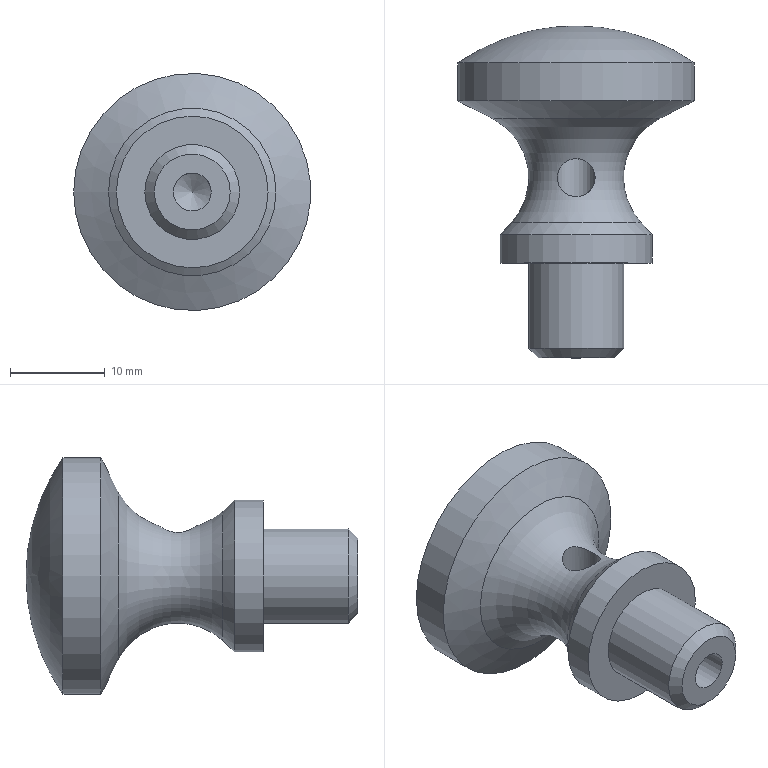Part | NX | 1 solid | 13 faces | box 25 x 35 x 25 mm | volume 6094 mm3 | cylinder 5 | cone 4 | plane 2 | torus 1 | sphere 1 | commonest cylinder face diameters 4 x2 10 x1 16 x1 25 x1
STEP:
#1=CARTESIAN_POINT('',(-8.832,6.242,0.));
#2=VERTEX_POINT('',#1);
#3=CARTESIAN_POINT('',(0.,6.242,0.));
#4=DIRECTION('',(0.,1.,0.));
#5=DIRECTION('',(-1.,0.,0.));
#6=AXIS2_PLACEMENT_3D('',#3,#4,#5);
#7=CIRCLE('',#6,8.832);
#8=EDGE_CURVE('',#2,#2,#7,.T.);
#9=ORIENTED_EDGE('',*,*,#8,.F.);
#10=EDGE_LOOP('',(#9));
#11=FACE_BOUND('',#10,.T.);
#12=CARTESIAN_POINT('',(-6.832,-4.721,0.));
#13=VERTEX_POINT('',#12);
#14=CARTESIAN_POINT('',(0.,-4.721,0.));
#15=DIRECTION('',(0.,1.,0.));
#16=DIRECTION('',(-1.,0.,0.));
#17=AXIS2_PLACEMENT_3D('',#14,#15,#16);
#18=CIRCLE('',#17,6.832);
#19=EDGE_CURVE('',#13,#13,#18,.T.);
#20=ORIENTED_EDGE('',*,*,#19,.T.);
#21=EDGE_LOOP('',(#20));
#22=FACE_BOUND('',#21,.T.);
#23=CARTESIAN_POINT('',(-1.589,-1.215,4.853));
#24=VERTEX_POINT('',#23);
#25=CARTESIAN_POINT('',(-1.589,-1.215,4.853));
#26=CARTESIAN_POINT('',(-1.713,-1.053,4.782));
#27=CARTESIAN_POINT('',(-1.814,-0.8679,4.715));
#28=CARTESIAN_POINT('',(-1.885,-0.6696,4.666));
#29=CARTESIAN_POINT('',(-1.955,-0.4701,4.617));
#30=CARTESIAN_POINT('',(-1.996,-0.2505,4.585));
#31=CARTESIAN_POINT('',(-2.,-0.03311,4.583));
#32=CARTESIAN_POINT('',(-2.003,0.1566,4.58));
#33=CARTESIAN_POINT('',(-1.978,0.3496,4.599));
#34=CARTESIAN_POINT('',(-1.929,0.5294,4.635));
#35=CARTESIAN_POINT('',(-1.881,0.704,4.669));
#36=CARTESIAN_POINT('',(-1.809,0.8707,4.719));
#37=CARTESIAN_POINT('',(-1.719,1.022,4.775));
#38=CARTESIAN_POINT('',(-1.614,1.198,4.84));
#39=CARTESIAN_POINT('',(-1.483,1.358,4.915));
#40=CARTESIAN_POINT('',(-1.331,1.493,4.987));
#41=CARTESIAN_POINT('',(-1.156,1.649,5.069));
#42=CARTESIAN_POINT('',(-0.9478,1.778,5.147));
#43=CARTESIAN_POINT('',(-0.7218,1.865,5.203));
#44=CARTESIAN_POINT('',(-0.5452,1.934,5.247));
#45=CARTESIAN_POINT('',(-0.3528,1.978,5.277));
#46=CARTESIAN_POINT('',(-0.1593,1.994,5.288));
#47=CARTESIAN_POINT('',(0.03459,2.009,5.298));
#48=CARTESIAN_POINT('',(0.2347,1.996,5.289));
#49=CARTESIAN_POINT('',(0.4232,1.955,5.261));
#50=CARTESIAN_POINT('',(0.6044,1.915,5.235));
#51=CARTESIAN_POINT('',(0.7795,1.851,5.193));
#52=CARTESIAN_POINT('',(0.9385,1.766,5.141));
#53=CARTESIAN_POINT('',(1.115,1.672,5.084));
#54=CARTESIAN_POINT('',(1.276,1.553,5.015));
#55=CARTESIAN_POINT('',(1.414,1.414,4.946));
#56=CARTESIAN_POINT('',(1.575,1.253,4.866));
#57=CARTESIAN_POINT('',(1.71,1.063,4.783));
#58=CARTESIAN_POINT('',(1.809,0.8526,4.717));
#59=CARTESIAN_POINT('',(1.89,0.6804,4.663));
#60=CARTESIAN_POINT('',(1.949,0.4907,4.62));
#61=CARTESIAN_POINT('',(1.978,0.2963,4.599));
#62=CARTESIAN_POINT('',(2.007,0.101,4.577));
#63=CARTESIAN_POINT('',(2.007,-0.1043,4.578));
#64=CARTESIAN_POINT('',(1.977,-0.2995,4.599));
#65=CARTESIAN_POINT('',(1.951,-0.4772,4.619));
#66=CARTESIAN_POINT('',(1.899,-0.651,4.657));
#67=CARTESIAN_POINT('',(1.828,-0.8105,4.704));
#68=CARTESIAN_POINT('',(1.751,-0.9862,4.757));
#69=CARTESIAN_POINT('',(1.648,-1.149,4.821));
#70=CARTESIAN_POINT('',(1.526,-1.292,4.888));
#71=CARTESIAN_POINT('',(1.382,-1.463,4.966));
#72=CARTESIAN_POINT('',(1.206,-1.611,5.049));
#73=CARTESIAN_POINT('',(1.01,-1.726,5.117));
#74=CARTESIAN_POINT('',(0.8381,-1.827,5.177));
#75=CARTESIAN_POINT('',(0.645,-1.904,5.228));
#76=CARTESIAN_POINT('',(0.444,-1.95,5.258));
#77=CARTESIAN_POINT('',(0.2421,-1.996,5.289));
#78=CARTESIAN_POINT('',(0.02612,-2.011,5.299));
#79=CARTESIAN_POINT('',(-0.1819,-1.992,5.286));
#80=CARTESIAN_POINT('',(-0.3686,-1.975,5.275));
#81=CARTESIAN_POINT('',(-0.5538,-1.931,5.245));
#82=CARTESIAN_POINT('',(-0.7243,-1.864,5.203));
#83=CARTESIAN_POINT('',(-0.9022,-1.795,5.159));
#84=CARTESIAN_POINT('',(-1.069,-1.701,5.1));
#85=CARTESIAN_POINT('',(-1.216,-1.588,5.038));
#86=CARTESIAN_POINT('',(-1.356,-1.481,4.978));
#87=CARTESIAN_POINT('',(-1.482,-1.355,4.914));
#88=CARTESIAN_POINT('',(-1.589,-1.215,4.853));
#89=B_SPLINE_CURVE_WITH_KNOTS('',3,(#25,#26,#27,#28,#29,#30,#31,#32,#33,#34,#35,#36,#37,#38,#39,#40,#41,#42,#43,#44,#45,#46,#47,#48,#49,#50,#51,#52,#53,#54,#55,#56,#57,#58,#59,#60,#61,#62,#63,#64,#65,#66,#67,#68,#69,#70,#71,#72,#73,#74,#75,#76,#77,#78,#79,#80,#81,#82,#83,#84,#85,#86,#87,#88),.UNSPECIFIED.,.T.,.F.,(1,3,3,3,3,3,3,3,3,3,3,3,3,3,3,3,3,3,3,3,3,3,3,1),(-0.04307,0.,0.05034,0.1012,0.1454,0.1882,0.2383,0.2964,0.3417,0.387,0.4305,0.4787,0.535,0.5809,0.6272,0.6692,0.7154,0.7706,0.8191,0.8679,0.9115,0.9569,1.,1.05),.UNSPECIFIED.);
#90=EDGE_CURVE('',#24,#24,#89,.T.);
#91=ORIENTED_EDGE('',*,*,#90,.T.);
#92=EDGE_LOOP('',(#91));
#93=FACE_BOUND('',#92,.T.);
#94=CARTESIAN_POINT('',(0.,0.,0.));
#95=DIRECTION('',(0.,1.,0.));
#96=DIRECTION('',(1.,0.,0.));
#97=AXIS2_PLACEMENT_3D('',#94,#95,#96);
#98=TOROIDAL_SURFACE('',#97,12.,7.);
#99=ADVANCED_FACE('',(#11,#22,#93),#98,.F.);
#100=CARTESIAN_POINT('',(-2.,-19.,0.));
#101=VERTEX_POINT('',#100);
#102=CARTESIAN_POINT('',(0.,-19.,0.));
#103=DIRECTION('',(0.,1.,0.));
#104=DIRECTION('',(-1.,0.,0.));
#105=AXIS2_PLACEMENT_3D('',#102,#103,#104);
#106=CIRCLE('',#105,2.);
#107=EDGE_CURVE('',#101,#101,#106,.T.);
#108=ORIENTED_EDGE('',*,*,#107,.T.);
#109=EDGE_LOOP('',(#108));
#110=FACE_BOUND('',#109,.T.);
#111=CARTESIAN_POINT('',(-4.,-19.,0.));
#112=VERTEX_POINT('',#111);
#113=CARTESIAN_POINT('',(0.,-19.,0.));
#114=DIRECTION('',(0.,1.,0.));
#115=DIRECTION('',(-1.,0.,0.));
#116=AXIS2_PLACEMENT_3D('',#113,#114,#115);
#117=CIRCLE('',#116,4.);
#118=EDGE_CURVE('',#112,#112,#117,.T.);
#119=ORIENTED_EDGE('',*,*,#118,.F.);
#120=EDGE_LOOP('',(#119));
#121=FACE_BOUND('',#120,.T.);
#122=CARTESIAN_POINT('',(-4.,-19.,0.));
#123=DIRECTION('',(0.,-1.,0.));
#124=DIRECTION('',(-1.,0.,0.));
#125=AXIS2_PLACEMENT_3D('',#122,#123,#124);
#126=PLANE('',#125);
#127=ADVANCED_FACE('',(#110,#121),#126,.T.);
#128=ORIENTED_EDGE('',*,*,#118,.T.);
#129=EDGE_LOOP('',(#128));
#130=FACE_BOUND('',#129,.T.);
#131=CARTESIAN_POINT('',(-5.,-18.,0.));
#132=VERTEX_POINT('',#131);
#133=CARTESIAN_POINT('',(0.,-18.,0.));
#134=DIRECTION('',(0.,1.,0.));
#135=DIRECTION('',(-1.,0.,0.));
#136=AXIS2_PLACEMENT_3D('',#133,#134,#135);
#137=CIRCLE('',#136,5.);
#138=EDGE_CURVE('',#132,#132,#137,.T.);
#139=ORIENTED_EDGE('',*,*,#138,.F.);
#140=EDGE_LOOP('',(#139));
#141=FACE_BOUND('',#140,.T.);
#142=CARTESIAN_POINT('',(0.,-18.,0.));
#143=DIRECTION('',(0.,1.,0.));
#144=DIRECTION('',(1.,0.,0.));
#145=AXIS2_PLACEMENT_3D('',#142,#143,#144);
#146=CONICAL_SURFACE('',#145,5.,45.);
#147=ADVANCED_FACE('',(#130,#141),#146,.T.);
#148=ORIENTED_EDGE('',*,*,#138,.T.);
#149=EDGE_LOOP('',(#148));
#150=FACE_BOUND('',#149,.T.);
#151=CARTESIAN_POINT('',(-5.,-9.,0.));
#152=VERTEX_POINT('',#151);
#153=CARTESIAN_POINT('',(0.,-9.,0.));
#154=DIRECTION('',(0.,1.,0.));
#155=DIRECTION('',(-1.,0.,0.));
#156=AXIS2_PLACEMENT_3D('',#153,#154,#155);
#157=CIRCLE('',#156,5.);
#158=EDGE_CURVE('',#152,#152,#157,.T.);
#159=ORIENTED_EDGE('',*,*,#158,.F.);
#160=EDGE_LOOP('',(#159));
#161=FACE_BOUND('',#160,.T.);
#162=CARTESIAN_POINT('',(0.,20.035,0.));
#163=DIRECTION('',(0.,1.,0.));
#164=DIRECTION('',(1.,0.,0.));
#165=AXIS2_PLACEMENT_3D('',#162,#163,#164);
#166=CYLINDRICAL_SURFACE('',#165,5.);
#167=ADVANCED_FACE('',(#150,#161),#166,.T.);
#168=ORIENTED_EDGE('',*,*,#158,.T.);
#169=EDGE_LOOP('',(#168));
#170=FACE_BOUND('',#169,.T.);
#171=CARTESIAN_POINT('',(-8.,-9.,0.));
#172=VERTEX_POINT('',#171);
#173=CARTESIAN_POINT('',(0.,-9.,0.));
#174=DIRECTION('',(0.,1.,0.));
#175=DIRECTION('',(-1.,0.,0.));
#176=AXIS2_PLACEMENT_3D('',#173,#174,#175);
#177=CIRCLE('',#176,8.);
#178=EDGE_CURVE('',#172,#172,#177,.T.);
#179=ORIENTED_EDGE('',*,*,#178,.F.);
#180=EDGE_LOOP('',(#179));
#181=FACE_BOUND('',#180,.T.);
#182=CARTESIAN_POINT('',(-8.,-9.,0.));
#183=DIRECTION('',(0.,-1.,0.));
#184=DIRECTION('',(-1.,0.,0.));
#185=AXIS2_PLACEMENT_3D('',#182,#183,#184);
#186=PLANE('',#185);
#187=ADVANCED_FACE('',(#170,#181),#186,.T.);
#188=ORIENTED_EDGE('',*,*,#178,.T.);
#189=EDGE_LOOP('',(#188));
#190=FACE_BOUND('',#189,.T.);
#191=CARTESIAN_POINT('',(-8.,-6.,0.));
#192=VERTEX_POINT('',#191);
#193=CARTESIAN_POINT('',(0.,-6.,0.));
#194=DIRECTION('',(0.,1.,0.));
#195=DIRECTION('',(-1.,0.,0.));
#196=AXIS2_PLACEMENT_3D('',#193,#194,#195);
#197=CIRCLE('',#196,8.);
#198=EDGE_CURVE('',#192,#192,#197,.T.);
#199=ORIENTED_EDGE('',*,*,#198,.F.);
#200=EDGE_LOOP('',(#199));
#201=FACE_BOUND('',#200,.T.);
#202=CARTESIAN_POINT('',(0.,20.035,0.));
#203=DIRECTION('',(0.,1.,0.));
#204=DIRECTION('',(1.,0.,0.));
#205=AXIS2_PLACEMENT_3D('',#202,#203,#204);
#206=CYLINDRICAL_SURFACE('',#205,8.);
#207=ADVANCED_FACE('',(#190,#201),#206,.T.);
#208=ORIENTED_EDGE('',*,*,#198,.T.);
#209=EDGE_LOOP('',(#208));
#210=FACE_BOUND('',#209,.T.);
#211=ORIENTED_EDGE('',*,*,#19,.F.);
#212=EDGE_LOOP('',(#211));
#213=FACE_BOUND('',#212,.T.);
#214=CARTESIAN_POINT('',(0.,-4.721,0.));
#215=DIRECTION('',(0.,-1.,0.));
#216=DIRECTION('',(-1.,0.,0.));
#217=AXIS2_PLACEMENT_3D('',#214,#215,#216);
#218=CONICAL_SURFACE('',#217,6.832,42.412);
#219=ADVANCED_FACE('',(#210,#213),#218,.T.);
#220=ORIENTED_EDGE('',*,*,#8,.T.);
#221=EDGE_LOOP('',(#220));
#222=FACE_BOUND('',#221,.T.);
#223=CARTESIAN_POINT('',(-12.5,8.104,0.));
#224=VERTEX_POINT('',#223);
#225=CARTESIAN_POINT('',(0.,8.104,0.));
#226=DIRECTION('',(0.,1.,0.));
#227=DIRECTION('',(-1.,0.,0.));
#228=AXIS2_PLACEMENT_3D('',#225,#226,#227);
#229=CIRCLE('',#228,12.5);
#230=EDGE_CURVE('',#224,#224,#229,.T.);
#231=ORIENTED_EDGE('',*,*,#230,.F.);
#232=EDGE_LOOP('',(#231));
#233=FACE_BOUND('',#232,.T.);
#234=CARTESIAN_POINT('',(0.,8.104,0.));
#235=DIRECTION('',(0.,1.,0.));
#236=DIRECTION('',(1.,0.,0.));
#237=AXIS2_PLACEMENT_3D('',#234,#235,#236);
#238=CONICAL_SURFACE('',#237,12.5,63.089);
#239=ADVANCED_FACE('',(#222,#233),#238,.T.);
#240=ORIENTED_EDGE('',*,*,#230,.T.);
#241=EDGE_LOOP('',(#240));
#242=FACE_BOUND('',#241,.T.);
#243=CARTESIAN_POINT('',(-12.5,12.104,0.));
#244=VERTEX_POINT('',#243);
#245=CARTESIAN_POINT('',(0.,12.104,0.));
#246=DIRECTION('',(0.,1.,0.));
#247=DIRECTION('',(-1.,0.,0.));
#248=AXIS2_PLACEMENT_3D('',#245,#246,#247);
#249=CIRCLE('',#248,12.5);
#250=EDGE_CURVE('',#244,#244,#249,.T.);
#251=ORIENTED_EDGE('',*,*,#250,.F.);
#252=EDGE_LOOP('',(#251));
#253=FACE_BOUND('',#252,.T.);
#254=CARTESIAN_POINT('',(0.,20.035,0.));
#255=DIRECTION('',(0.,1.,0.));
#256=DIRECTION('',(1.,0.,0.));
#257=AXIS2_PLACEMENT_3D('',#254,#255,#256);
#258=CYLINDRICAL_SURFACE('',#257,12.5);
#259=ADVANCED_FACE('',(#242,#253),#258,.T.);
#260=ORIENTED_EDGE('',*,*,#250,.T.);
#261=EDGE_LOOP('',(#260));
#262=FACE_OUTER_BOUND('',#261,.T.);
#263=CARTESIAN_POINT('',(0.,-6.,0.));
#264=DIRECTION('',(0.,1.,0.));
#265=DIRECTION('',(-1.,0.,0.));
#266=AXIS2_PLACEMENT_3D('',#263,#264,#265);
#267=SPHERICAL_SURFACE('',#266,22.);
#268=ADVANCED_FACE('',(#262),#267,.T.);
#269=CARTESIAN_POINT('',(2.,0.,0.));
#270=VERTEX_POINT('',#269);
#271=CARTESIAN_POINT('',(-2.,0.,0.));
#272=VERTEX_POINT('',#271);
#273=CARTESIAN_POINT('',(0.,0.,0.));
#274=DIRECTION('',(0.,-0.7071,0.7071));
#275=DIRECTION('',(0.,-0.7071,-0.7071));
#276=AXIS2_PLACEMENT_3D('',#273,#274,#275);
#277=ELLIPSE('',#276,2.828,2.);
#278=EDGE_CURVE('',#270,#272,#277,.T.);
#279=ORIENTED_EDGE('',*,*,#278,.F.);
#280=CARTESIAN_POINT('',(0.,0.,0.));
#281=DIRECTION('',(0.,0.7071,0.7071));
#282=DIRECTION('',(0.,0.7071,-0.7071));
#283=AXIS2_PLACEMENT_3D('',#280,#281,#282);
#284=ELLIPSE('',#283,2.828,2.);
#285=EDGE_CURVE('',#272,#270,#284,.T.);
#286=ORIENTED_EDGE('',*,*,#285,.F.);
#287=EDGE_LOOP('',(#279,#286));
#288=FACE_BOUND('',#287,.T.);
#289=ORIENTED_EDGE('',*,*,#90,.F.);
#290=EDGE_LOOP('',(#289));
#291=FACE_BOUND('',#290,.T.);
#292=CARTESIAN_POINT('',(0.,0.,20.));
#293=DIRECTION('',(0.,0.,-1.));
#294=DIRECTION('',(1.,0.,0.));
#295=AXIS2_PLACEMENT_3D('',#292,#293,#294);
#296=CYLINDRICAL_SURFACE('',#295,2.);
#297=ADVANCED_FACE('',(#288,#291),#296,.F.);
#298=CARTESIAN_POINT('',(-2.,4.333,0.));
#299=VERTEX_POINT('',#298);
#300=CARTESIAN_POINT('',(0.,4.333,0.));
#301=DIRECTION('',(0.,-1.,0.));
#302=DIRECTION('',(-1.,0.,0.));
#303=AXIS2_PLACEMENT_3D('',#300,#301,#302);
#304=CIRCLE('',#303,2.);
#305=EDGE_CURVE('',#299,#299,#304,.T.);
#306=ORIENTED_EDGE('',*,*,#305,.T.);
#307=EDGE_LOOP('',(#306));
#308=FACE_BOUND('',#307,.T.);
#309=CARTESIAN_POINT('',(0.,5.535,0.));
#310=VERTEX_POINT('',#309);
#311=VERTEX_LOOP('',#310);
#312=FACE_BOUND('',#311,.T.);
#313=CARTESIAN_POINT('',(0.,4.333,0.));
#314=DIRECTION('',(0.,-1.,0.));
#315=DIRECTION('',(-1.,0.,0.));
#316=AXIS2_PLACEMENT_3D('',#313,#314,#315);
#317=CONICAL_SURFACE('',#316,2.,59.);
#318=ADVANCED_FACE('',(#308,#312),#317,.F.);
#319=ORIENTED_EDGE('',*,*,#278,.T.);
#320=ORIENTED_EDGE('',*,*,#285,.T.);
#321=EDGE_LOOP('',(#319,#320));
#322=FACE_BOUND('',#321,.T.);
#323=ORIENTED_EDGE('',*,*,#305,.F.);
#324=EDGE_LOOP('',(#323));
#325=FACE_BOUND('',#324,.T.);
#326=ORIENTED_EDGE('',*,*,#107,.F.);
#327=EDGE_LOOP('',(#326));
#328=FACE_BOUND('',#327,.T.);
#329=CARTESIAN_POINT('',(0.,-19.,0.));
#330=DIRECTION('',(0.,1.,0.));
#331=DIRECTION('',(1.,0.,0.));
#332=AXIS2_PLACEMENT_3D('',#329,#330,#331);
#333=CYLINDRICAL_SURFACE('',#332,2.);
#334=ADVANCED_FACE('',(#322,#325,#328),#333,.F.);
#335=CLOSED_SHELL('',(#99,#127,#147,#167,#187,#207,#219,#239,#259,#268,#297,#318,#334));
#336=MANIFOLD_SOLID_BREP('',#335);
#337=(LENGTH_UNIT()NAMED_UNIT(*)SI_UNIT(.MILLI.,.METRE.));
#338=UNCERTAINTY_MEASURE_WITH_UNIT(LENGTH_MEASURE(0.0508),#337,'','');
#339=(NAMED_UNIT(*)PLANE_ANGLE_UNIT()SI_UNIT($,.RADIAN.));
#340=PLANE_ANGLE_MEASURE_WITH_UNIT(PLANE_ANGLE_MEASURE(0.01745),#339);
#341=DIMENSIONAL_EXPONENTS(0.,0.,0.,0.,0.,0.,0.);
#342=(CONVERSION_BASED_UNIT('DEGREE',#340)NAMED_UNIT(#341)PLANE_ANGLE_UNIT());
#343=(NAMED_UNIT(*)SI_UNIT($,.STERADIAN.)SOLID_ANGLE_UNIT());
#344=(GEOMETRIC_REPRESENTATION_CONTEXT(3)GLOBAL_UNCERTAINTY_ASSIGNED_CONTEXT((#338))GLOBAL_UNIT_ASSIGNED_CONTEXT((#337,#342,#343))REPRESENTATION_CONTEXT('',''));
#345=ADVANCED_BREP_SHAPE_REPRESENTATION('',(#336),#344);